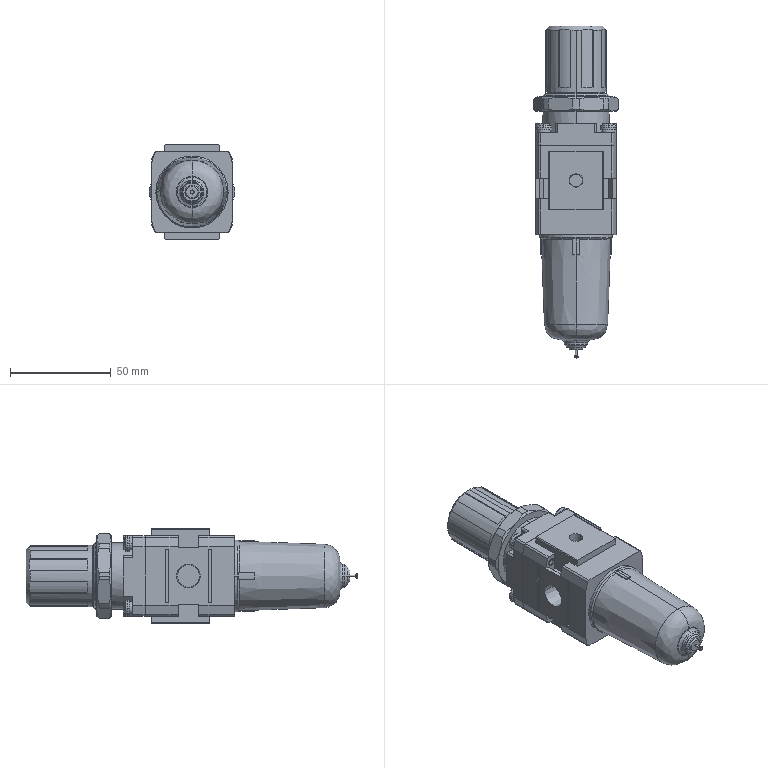Part | STEP file | 1 solid | 397 faces | box 42.5 x 165.1 x 47 mm | volume 170625 mm3 | plane 248 | cylinder 89 | cone 36 | spline 16 | other 8 | commonest cylinder face diameters 2 x21 42.5 x9 3.242 x8 6.6 x8 8 x8 29.5 x8